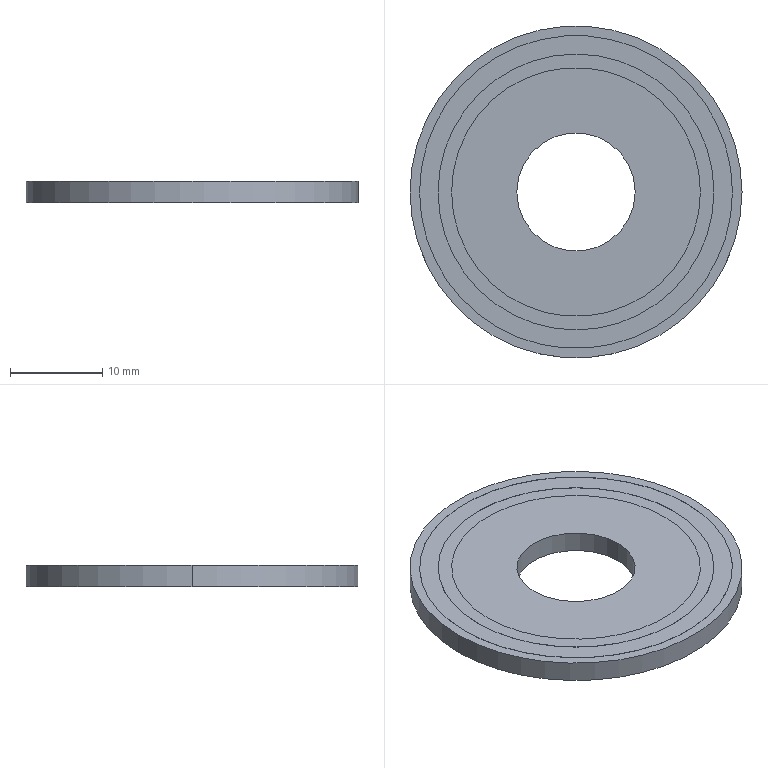Part | STEP file | 2 solids | 18 faces | box 35.9 x 35.9 x 2.3 mm | volume 2028 mm3 | cylinder 12 | plane 6 | commonest cylinder face diameters 26.9 x4 12.8 x2 29.83 x2 33.83 x2 35.9 x2
STEP:
#1=CARTESIAN_POINT('',(0.,0.,0.));
#2=DIRECTION('',(0.,0.,1.));
#3=DIRECTION('',(1.,0.,0.));
#4=AXIS2_PLACEMENT_3D('',#1,#2,#3);
#5=CARTESIAN_POINT('',(-13.45,0.,0.));
#6=VERTEX_POINT('',#5);
#7=CARTESIAN_POINT('',(-13.45,0.,2.3));
#8=VERTEX_POINT('',#7);
#9=CARTESIAN_POINT('',(-13.45,0.,-0.01));
#10=DIRECTION('',(0.,0.,1.));
#11=VECTOR('',#10,1.);
#12=LINE('',#9,#11);
#13=CARTESIAN_POINT('',(0.,0.,-0.01));
#14=DIRECTION('',(0.,0.,1.));
#15=DIRECTION('',(1.,0.,0.));
#16=AXIS2_PLACEMENT_3D('',#13,#14,#15);
#17=CYLINDRICAL_SURFACE('',#16,13.45);
#18=CARTESIAN_POINT('',(3.142,0.));
#19=DIRECTION('',(0.,1.));
#20=VECTOR('',#19,1.);
#21=LINE('',#18,#20);
#22=(GEOMETRIC_REPRESENTATION_CONTEXT(2)PARAMETRIC_REPRESENTATION_CONTEXT()REPRESENTATION_CONTEXT('',''));
#23=DEFINITIONAL_REPRESENTATION('',(#21),#22);
#24=PCURVE('',#17,#23);
#25=CARTESIAN_POINT('',(0.,0.,-0.01));
#26=DIRECTION('',(0.,0.,1.));
#27=DIRECTION('',(1.,0.,0.));
#28=AXIS2_PLACEMENT_3D('',#25,#26,#27);
#29=CYLINDRICAL_SURFACE('',#28,13.45);
#30=CARTESIAN_POINT('',(3.142,0.));
#31=DIRECTION('',(0.,1.));
#32=VECTOR('',#31,1.);
#33=LINE('',#30,#32);
#34=(GEOMETRIC_REPRESENTATION_CONTEXT(2)PARAMETRIC_REPRESENTATION_CONTEXT()REPRESENTATION_CONTEXT('',''));
#35=DEFINITIONAL_REPRESENTATION('',(#33),#34);
#36=PCURVE('',#29,#35);
#37=SURFACE_CURVE('',#12,(#24,#36),.PCURVE_S1.);
#38=EDGE_CURVE('',#6,#8,#37,.T.);
#39=ORIENTED_EDGE('',*,*,#38,.F.);
#40=CARTESIAN_POINT('',(13.45,0.,0.));
#41=VERTEX_POINT('',#40);
#42=CARTESIAN_POINT('',(0.,0.,0.));
#43=DIRECTION('',(0.,0.,1.));
#44=DIRECTION('',(1.,0.,0.));
#45=AXIS2_PLACEMENT_3D('',#42,#43,#44);
#46=CIRCLE('',#45,13.45);
#47=CARTESIAN_POINT('',(0.,0.01));
#48=DIRECTION('',(1.,0.));
#49=VECTOR('',#48,1.);
#50=LINE('',#47,#49);
#51=(GEOMETRIC_REPRESENTATION_CONTEXT(2)PARAMETRIC_REPRESENTATION_CONTEXT()REPRESENTATION_CONTEXT('',''));
#52=DEFINITIONAL_REPRESENTATION('',(#50),#51);
#53=PCURVE('',#17,#52);
#54=CARTESIAN_POINT('',(0.,0.,0.));
#55=DIRECTION('',(0.,0.,1.));
#56=DIRECTION('',(1.,0.,0.));
#57=AXIS2_PLACEMENT_3D('',#54,#55,#56);
#58=PLANE('',#57);
#59=CARTESIAN_POINT('',(0.,0.));
#60=DIRECTION('',(1.,0.));
#61=AXIS2_PLACEMENT_2D('',#59,#60);
#62=CIRCLE('',#61,13.45);
#63=(GEOMETRIC_REPRESENTATION_CONTEXT(2)PARAMETRIC_REPRESENTATION_CONTEXT()REPRESENTATION_CONTEXT('',''));
#64=DEFINITIONAL_REPRESENTATION('',(#62),#63);
#65=PCURVE('',#58,#64);
#66=SURFACE_CURVE('',#46,(#53,#65),.PCURVE_S1.);
#67=EDGE_CURVE('',#6,#41,#66,.T.);
#68=ORIENTED_EDGE('',*,*,#67,.T.);
#69=CARTESIAN_POINT('',(13.45,0.,2.3));
#70=VERTEX_POINT('',#69);
#71=CARTESIAN_POINT('',(13.45,0.,-0.01));
#72=DIRECTION('',(0.,0.,1.));
#73=VECTOR('',#72,1.);
#74=LINE('',#71,#73);
#75=CARTESIAN_POINT('',(6.283,0.));
#76=DIRECTION('',(0.,1.));
#77=VECTOR('',#76,1.);
#78=LINE('',#75,#77);
#79=(GEOMETRIC_REPRESENTATION_CONTEXT(2)PARAMETRIC_REPRESENTATION_CONTEXT()REPRESENTATION_CONTEXT('',''));
#80=DEFINITIONAL_REPRESENTATION('',(#78),#79);
#81=PCURVE('',#17,#80);
#82=CARTESIAN_POINT('',(0.,0.));
#83=DIRECTION('',(0.,1.));
#84=VECTOR('',#83,1.);
#85=LINE('',#82,#84);
#86=(GEOMETRIC_REPRESENTATION_CONTEXT(2)PARAMETRIC_REPRESENTATION_CONTEXT()REPRESENTATION_CONTEXT('',''));
#87=DEFINITIONAL_REPRESENTATION('',(#85),#86);
#88=PCURVE('',#29,#87);
#89=SURFACE_CURVE('',#74,(#81,#88),.PCURVE_S1.);
#90=EDGE_CURVE('',#41,#70,#89,.T.);
#91=ORIENTED_EDGE('',*,*,#90,.T.);
#92=CARTESIAN_POINT('',(0.,0.,2.3));
#93=DIRECTION('',(0.,0.,1.));
#94=DIRECTION('',(1.,0.,0.));
#95=AXIS2_PLACEMENT_3D('',#92,#93,#94);
#96=CIRCLE('',#95,13.45);
#97=CARTESIAN_POINT('',(0.,2.31));
#98=DIRECTION('',(1.,0.));
#99=VECTOR('',#98,1.);
#100=LINE('',#97,#99);
#101=(GEOMETRIC_REPRESENTATION_CONTEXT(2)PARAMETRIC_REPRESENTATION_CONTEXT()REPRESENTATION_CONTEXT('',''));
#102=DEFINITIONAL_REPRESENTATION('',(#100),#101);
#103=PCURVE('',#17,#102);
#104=CARTESIAN_POINT('',(0.,0.,2.3));
#105=DIRECTION('',(0.,0.,1.));
#106=DIRECTION('',(1.,0.,0.));
#107=AXIS2_PLACEMENT_3D('',#104,#105,#106);
#108=PLANE('',#107);
#109=CARTESIAN_POINT('',(0.,0.));
#110=DIRECTION('',(1.,0.));
#111=AXIS2_PLACEMENT_2D('',#109,#110);
#112=CIRCLE('',#111,13.45);
#113=(GEOMETRIC_REPRESENTATION_CONTEXT(2)PARAMETRIC_REPRESENTATION_CONTEXT()REPRESENTATION_CONTEXT('',''));
#114=DEFINITIONAL_REPRESENTATION('',(#112),#113);
#115=PCURVE('',#108,#114);
#116=SURFACE_CURVE('',#96,(#103,#115),.PCURVE_S1.);
#117=EDGE_CURVE('',#8,#70,#116,.T.);
#118=ORIENTED_EDGE('',*,*,#117,.F.);
#119=EDGE_LOOP('',(#39,#68,#91,#118));
#120=FACE_BOUND('',#119,.T.);
#121=ADVANCED_FACE('',(#120),#17,.T.);
#122=CARTESIAN_POINT('',(6.4,0.,0.));
#123=VERTEX_POINT('',#122);
#124=CARTESIAN_POINT('',(-6.4,0.,0.));
#125=VERTEX_POINT('',#124);
#126=CARTESIAN_POINT('',(0.,0.,0.));
#127=DIRECTION('',(0.,0.,1.));
#128=DIRECTION('',(1.,0.,0.));
#129=AXIS2_PLACEMENT_3D('',#126,#127,#128);
#130=CIRCLE('',#129,6.4);
#131=CARTESIAN_POINT('',(0.,0.,2.3));
#132=DIRECTION('',(0.,0.,-1.));
#133=DIRECTION('',(-1.,0.,0.));
#134=AXIS2_PLACEMENT_3D('',#131,#132,#133);
#135=CYLINDRICAL_SURFACE('',#134,6.4);
#136=CARTESIAN_POINT('',(3.142,2.3));
#137=DIRECTION('',(-1.,0.));
#138=VECTOR('',#137,1.);
#139=LINE('',#136,#138);
#140=(GEOMETRIC_REPRESENTATION_CONTEXT(2)PARAMETRIC_REPRESENTATION_CONTEXT()REPRESENTATION_CONTEXT('',''));
#141=DEFINITIONAL_REPRESENTATION('',(#139),#140);
#142=PCURVE('',#135,#141);
#143=CARTESIAN_POINT('',(0.,0.));
#144=DIRECTION('',(1.,0.));
#145=AXIS2_PLACEMENT_2D('',#143,#144);
#146=CIRCLE('',#145,6.4);
#147=(GEOMETRIC_REPRESENTATION_CONTEXT(2)PARAMETRIC_REPRESENTATION_CONTEXT()REPRESENTATION_CONTEXT('',''));
#148=DEFINITIONAL_REPRESENTATION('',(#146),#147);
#149=PCURVE('',#58,#148);
#150=SURFACE_CURVE('',#130,(#142,#149),.PCURVE_S1.);
#151=EDGE_CURVE('',#123,#125,#150,.T.);
#152=ORIENTED_EDGE('',*,*,#151,.T.);
#153=CARTESIAN_POINT('',(-6.4,0.,2.3));
#154=VERTEX_POINT('',#153);
#155=CARTESIAN_POINT('',(-6.4,0.,2.3));
#156=DIRECTION('',(0.,0.,-1.));
#157=VECTOR('',#156,1.);
#158=LINE('',#155,#157);
#159=CARTESIAN_POINT('',(0.,0.));
#160=DIRECTION('',(0.,1.));
#161=VECTOR('',#160,1.);
#162=LINE('',#159,#161);
#163=(GEOMETRIC_REPRESENTATION_CONTEXT(2)PARAMETRIC_REPRESENTATION_CONTEXT()REPRESENTATION_CONTEXT('',''));
#164=DEFINITIONAL_REPRESENTATION('',(#162),#163);
#165=PCURVE('',#135,#164);
#166=CARTESIAN_POINT('',(0.,0.,2.3));
#167=DIRECTION('',(0.,0.,-1.));
#168=DIRECTION('',(-1.,0.,0.));
#169=AXIS2_PLACEMENT_3D('',#166,#167,#168);
#170=CYLINDRICAL_SURFACE('',#169,6.4);
#171=CARTESIAN_POINT('',(6.283,0.));
#172=DIRECTION('',(0.,1.));
#173=VECTOR('',#172,1.);
#174=LINE('',#171,#173);
#175=(GEOMETRIC_REPRESENTATION_CONTEXT(2)PARAMETRIC_REPRESENTATION_CONTEXT()REPRESENTATION_CONTEXT('',''));
#176=DEFINITIONAL_REPRESENTATION('',(#174),#175);
#177=PCURVE('',#170,#176);
#178=SURFACE_CURVE('',#158,(#165,#177),.PCURVE_S1.);
#179=EDGE_CURVE('',#154,#125,#178,.T.);
#180=ORIENTED_EDGE('',*,*,#179,.F.);
#181=CARTESIAN_POINT('',(6.4,0.,2.3));
#182=VERTEX_POINT('',#181);
#183=CARTESIAN_POINT('',(0.,0.,2.3));
#184=DIRECTION('',(0.,0.,1.));
#185=DIRECTION('',(1.,0.,0.));
#186=AXIS2_PLACEMENT_3D('',#183,#184,#185);
#187=CIRCLE('',#186,6.4);
#188=CARTESIAN_POINT('',(3.142,0.));
#189=DIRECTION('',(-1.,0.));
#190=VECTOR('',#189,1.);
#191=LINE('',#188,#190);
#192=(GEOMETRIC_REPRESENTATION_CONTEXT(2)PARAMETRIC_REPRESENTATION_CONTEXT()REPRESENTATION_CONTEXT('',''));
#193=DEFINITIONAL_REPRESENTATION('',(#191),#192);
#194=PCURVE('',#135,#193);
#195=CARTESIAN_POINT('',(0.,0.));
#196=DIRECTION('',(1.,0.));
#197=AXIS2_PLACEMENT_2D('',#195,#196);
#198=CIRCLE('',#197,6.4);
#199=(GEOMETRIC_REPRESENTATION_CONTEXT(2)PARAMETRIC_REPRESENTATION_CONTEXT()REPRESENTATION_CONTEXT('',''));
#200=DEFINITIONAL_REPRESENTATION('',(#198),#199);
#201=PCURVE('',#108,#200);
#202=SURFACE_CURVE('',#187,(#194,#201),.PCURVE_S1.);
#203=EDGE_CURVE('',#182,#154,#202,.T.);
#204=ORIENTED_EDGE('',*,*,#203,.F.);
#205=CARTESIAN_POINT('',(6.4,0.,2.3));
#206=DIRECTION('',(0.,0.,-1.));
#207=VECTOR('',#206,1.);
#208=LINE('',#205,#207);
#209=CARTESIAN_POINT('',(3.142,0.));
#210=DIRECTION('',(0.,1.));
#211=VECTOR('',#210,1.);
#212=LINE('',#209,#211);
#213=(GEOMETRIC_REPRESENTATION_CONTEXT(2)PARAMETRIC_REPRESENTATION_CONTEXT()REPRESENTATION_CONTEXT('',''));
#214=DEFINITIONAL_REPRESENTATION('',(#212),#213);
#215=PCURVE('',#135,#214);
#216=CARTESIAN_POINT('',(3.142,0.));
#217=DIRECTION('',(0.,1.));
#218=VECTOR('',#217,1.);
#219=LINE('',#216,#218);
#220=(GEOMETRIC_REPRESENTATION_CONTEXT(2)PARAMETRIC_REPRESENTATION_CONTEXT()REPRESENTATION_CONTEXT('',''));
#221=DEFINITIONAL_REPRESENTATION('',(#219),#220);
#222=PCURVE('',#170,#221);
#223=SURFACE_CURVE('',#208,(#215,#222),.PCURVE_S1.);
#224=EDGE_CURVE('',#182,#123,#223,.T.);
#225=ORIENTED_EDGE('',*,*,#224,.T.);
#226=EDGE_LOOP('',(#152,#180,#204,#225));
#227=FACE_BOUND('',#226,.F.);
#228=ADVANCED_FACE('',(#227),#135,.F.);
#229=CARTESIAN_POINT('',(0.,0.,0.));
#230=DIRECTION('',(0.,0.,1.));
#231=DIRECTION('',(1.,0.,0.));
#232=AXIS2_PLACEMENT_3D('',#229,#230,#231);
#233=CIRCLE('',#232,13.45);
#234=CARTESIAN_POINT('',(0.,0.));
#235=DIRECTION('',(1.,0.));
#236=AXIS2_PLACEMENT_2D('',#234,#235);
#237=CIRCLE('',#236,13.45);
#238=(GEOMETRIC_REPRESENTATION_CONTEXT(2)PARAMETRIC_REPRESENTATION_CONTEXT()REPRESENTATION_CONTEXT('',''));
#239=DEFINITIONAL_REPRESENTATION('',(#237),#238);
#240=PCURVE('',#58,#239);
#241=CARTESIAN_POINT('',(0.,0.01));
#242=DIRECTION('',(1.,0.));
#243=VECTOR('',#242,1.);
#244=LINE('',#241,#243);
#245=(GEOMETRIC_REPRESENTATION_CONTEXT(2)PARAMETRIC_REPRESENTATION_CONTEXT()REPRESENTATION_CONTEXT('',''));
#246=DEFINITIONAL_REPRESENTATION('',(#244),#245);
#247=PCURVE('',#29,#246);
#248=SURFACE_CURVE('',#233,(#240,#247),.PCURVE_S1.);
#249=EDGE_CURVE('',#41,#6,#248,.T.);
#250=ORIENTED_EDGE('',*,*,#249,.F.);
#251=ORIENTED_EDGE('',*,*,#67,.F.);
#252=EDGE_LOOP('',(#250,#251));
#253=FACE_BOUND('',#252,.T.);
#254=CARTESIAN_POINT('',(0.,0.,0.));
#255=DIRECTION('',(0.,0.,1.));
#256=DIRECTION('',(1.,0.,0.));
#257=AXIS2_PLACEMENT_3D('',#254,#255,#256);
#258=CIRCLE('',#257,6.4);
#259=CARTESIAN_POINT('',(0.,0.));
#260=DIRECTION('',(1.,0.));
#261=AXIS2_PLACEMENT_2D('',#259,#260);
#262=CIRCLE('',#261,6.4);
#263=(GEOMETRIC_REPRESENTATION_CONTEXT(2)PARAMETRIC_REPRESENTATION_CONTEXT()REPRESENTATION_CONTEXT('',''));
#264=DEFINITIONAL_REPRESENTATION('',(#262),#263);
#265=PCURVE('',#58,#264);
#266=CARTESIAN_POINT('',(9.425,2.3));
#267=DIRECTION('',(-1.,0.));
#268=VECTOR('',#267,1.);
#269=LINE('',#266,#268);
#270=(GEOMETRIC_REPRESENTATION_CONTEXT(2)PARAMETRIC_REPRESENTATION_CONTEXT()REPRESENTATION_CONTEXT('',''));
#271=DEFINITIONAL_REPRESENTATION('',(#269),#270);
#272=PCURVE('',#170,#271);
#273=SURFACE_CURVE('',#258,(#265,#272),.PCURVE_S1.);
#274=EDGE_CURVE('',#125,#123,#273,.T.);
#275=ORIENTED_EDGE('',*,*,#274,.T.);
#276=ORIENTED_EDGE('',*,*,#151,.T.);
#277=EDGE_LOOP('',(#275,#276));
#278=FACE_BOUND('',#277,.T.);
#279=ADVANCED_FACE('',(#253,#278),#58,.F.);
#280=CARTESIAN_POINT('',(0.,0.,2.3));
#281=DIRECTION('',(0.,0.,1.));
#282=DIRECTION('',(1.,0.,0.));
#283=AXIS2_PLACEMENT_3D('',#280,#281,#282);
#284=CIRCLE('',#283,13.45);
#285=CARTESIAN_POINT('',(0.,0.));
#286=DIRECTION('',(1.,0.));
#287=AXIS2_PLACEMENT_2D('',#285,#286);
#288=CIRCLE('',#287,13.45);
#289=(GEOMETRIC_REPRESENTATION_CONTEXT(2)PARAMETRIC_REPRESENTATION_CONTEXT()REPRESENTATION_CONTEXT('',''));
#290=DEFINITIONAL_REPRESENTATION('',(#288),#289);
#291=PCURVE('',#108,#290);
#292=CARTESIAN_POINT('',(0.,2.31));
#293=DIRECTION('',(1.,0.));
#294=VECTOR('',#293,1.);
#295=LINE('',#292,#294);
#296=(GEOMETRIC_REPRESENTATION_CONTEXT(2)PARAMETRIC_REPRESENTATION_CONTEXT()REPRESENTATION_CONTEXT('',''));
#297=DEFINITIONAL_REPRESENTATION('',(#295),#296);
#298=PCURVE('',#29,#297);
#299=SURFACE_CURVE('',#284,(#291,#298),.PCURVE_S1.);
#300=EDGE_CURVE('',#70,#8,#299,.T.);
#301=ORIENTED_EDGE('',*,*,#300,.T.);
#302=ORIENTED_EDGE('',*,*,#117,.T.);
#303=EDGE_LOOP('',(#301,#302));
#304=FACE_BOUND('',#303,.T.);
#305=CARTESIAN_POINT('',(0.,0.,2.3));
#306=DIRECTION('',(0.,0.,1.));
#307=DIRECTION('',(1.,0.,0.));
#308=AXIS2_PLACEMENT_3D('',#305,#306,#307);
#309=CIRCLE('',#308,6.4);
#310=CARTESIAN_POINT('',(0.,0.));
#311=DIRECTION('',(1.,0.));
#312=AXIS2_PLACEMENT_2D('',#310,#311);
#313=CIRCLE('',#312,6.4);
#314=(GEOMETRIC_REPRESENTATION_CONTEXT(2)PARAMETRIC_REPRESENTATION_CONTEXT()REPRESENTATION_CONTEXT('',''));
#315=DEFINITIONAL_REPRESENTATION('',(#313),#314);
#316=PCURVE('',#108,#315);
#317=CARTESIAN_POINT('',(9.425,0.));
#318=DIRECTION('',(-1.,0.));
#319=VECTOR('',#318,1.);
#320=LINE('',#317,#319);
#321=(GEOMETRIC_REPRESENTATION_CONTEXT(2)PARAMETRIC_REPRESENTATION_CONTEXT()REPRESENTATION_CONTEXT('',''));
#322=DEFINITIONAL_REPRESENTATION('',(#320),#321);
#323=PCURVE('',#170,#322);
#324=SURFACE_CURVE('',#309,(#316,#323),.PCURVE_S1.);
#325=EDGE_CURVE('',#154,#182,#324,.T.);
#326=ORIENTED_EDGE('',*,*,#325,.F.);
#327=ORIENTED_EDGE('',*,*,#203,.F.);
#328=EDGE_LOOP('',(#326,#327));
#329=FACE_BOUND('',#328,.T.);
#330=ADVANCED_FACE('',(#304,#329),#108,.T.);
#331=ORIENTED_EDGE('',*,*,#249,.T.);
#332=ORIENTED_EDGE('',*,*,#38,.T.);
#333=ORIENTED_EDGE('',*,*,#300,.F.);
#334=ORIENTED_EDGE('',*,*,#90,.F.);
#335=EDGE_LOOP('',(#331,#332,#333,#334));
#336=FACE_BOUND('',#335,.T.);
#337=ADVANCED_FACE('',(#336),#29,.T.);
#338=ORIENTED_EDGE('',*,*,#179,.T.);
#339=ORIENTED_EDGE('',*,*,#274,.T.);
#340=ORIENTED_EDGE('',*,*,#224,.F.);
#341=ORIENTED_EDGE('',*,*,#325,.F.);
#342=EDGE_LOOP('',(#338,#339,#340,#341));
#343=FACE_BOUND('',#342,.F.);
#344=ADVANCED_FACE('',(#343),#170,.F.);
#345=CLOSED_SHELL('',(#121,#228,#279,#330,#337,#344));
#346=MANIFOLD_SOLID_BREP('',#345);
#347=CARTESIAN_POINT('',(-14.915,0.,2.28));
#348=VERTEX_POINT('',#347);
#349=CARTESIAN_POINT('',(-14.915,0.,2.3));
#350=VERTEX_POINT('',#349);
#351=CARTESIAN_POINT('',(-14.915,0.,2.28));
#352=DIRECTION('',(0.,0.,1.));
#353=VECTOR('',#352,1.);
#354=LINE('',#351,#353);
#355=CARTESIAN_POINT('',(0.,0.,2.28));
#356=DIRECTION('',(0.,0.,1.));
#357=DIRECTION('',(1.,0.,0.));
#358=AXIS2_PLACEMENT_3D('',#355,#356,#357);
#359=CYLINDRICAL_SURFACE('',#358,14.915);
#360=CARTESIAN_POINT('',(3.142,0.));
#361=DIRECTION('',(0.,1.));
#362=VECTOR('',#361,1.);
#363=LINE('',#360,#362);
#364=(GEOMETRIC_REPRESENTATION_CONTEXT(2)PARAMETRIC_REPRESENTATION_CONTEXT()REPRESENTATION_CONTEXT('',''));
#365=DEFINITIONAL_REPRESENTATION('',(#363),#364);
#366=PCURVE('',#359,#365);
#367=CARTESIAN_POINT('',(0.,0.,2.28));
#368=DIRECTION('',(0.,0.,1.));
#369=DIRECTION('',(1.,0.,0.));
#370=AXIS2_PLACEMENT_3D('',#367,#368,#369);
#371=CYLINDRICAL_SURFACE('',#370,14.915);
#372=CARTESIAN_POINT('',(3.142,0.));
#373=DIRECTION('',(0.,1.));
#374=VECTOR('',#373,1.);
#375=LINE('',#372,#374);
#376=(GEOMETRIC_REPRESENTATION_CONTEXT(2)PARAMETRIC_REPRESENTATION_CONTEXT()REPRESENTATION_CONTEXT('',''));
#377=DEFINITIONAL_REPRESENTATION('',(#375),#376);
#378=PCURVE('',#371,#377);
#379=SURFACE_CURVE('',#354,(#366,#378),.PCURVE_S1.);
#380=EDGE_CURVE('',#348,#350,#379,.T.);
#381=ORIENTED_EDGE('',*,*,#380,.F.);
#382=CARTESIAN_POINT('',(14.915,0.,2.28));
#383=VERTEX_POINT('',#382);
#384=CARTESIAN_POINT('',(0.,0.,2.28));
#385=DIRECTION('',(0.,0.,1.));
#386=DIRECTION('',(1.,0.,0.));
#387=AXIS2_PLACEMENT_3D('',#384,#385,#386);
#388=CIRCLE('',#387,14.915);
#389=CARTESIAN_POINT('',(0.,0.));
#390=DIRECTION('',(1.,0.));
#391=VECTOR('',#390,1.);
#392=LINE('',#389,#391);
#393=(GEOMETRIC_REPRESENTATION_CONTEXT(2)PARAMETRIC_REPRESENTATION_CONTEXT()REPRESENTATION_CONTEXT('',''));
#394=DEFINITIONAL_REPRESENTATION('',(#392),#393);
#395=PCURVE('',#359,#394);
#396=CARTESIAN_POINT('',(0.,0.,2.28));
#397=DIRECTION('',(0.,0.,1.));
#398=DIRECTION('',(1.,0.,0.));
#399=AXIS2_PLACEMENT_3D('',#396,#397,#398);
#400=PLANE('',#399);
#401=CARTESIAN_POINT('',(0.,0.));
#402=DIRECTION('',(1.,0.));
#403=AXIS2_PLACEMENT_2D('',#401,#402);
#404=CIRCLE('',#403,14.915);
#405=(GEOMETRIC_REPRESENTATION_CONTEXT(2)PARAMETRIC_REPRESENTATION_CONTEXT()REPRESENTATION_CONTEXT('',''));
#406=DEFINITIONAL_REPRESENTATION('',(#404),#405);
#407=PCURVE('',#400,#406);
#408=SURFACE_CURVE('',#388,(#395,#407),.PCURVE_S1.);
#409=EDGE_CURVE('',#348,#383,#408,.T.);
#410=ORIENTED_EDGE('',*,*,#409,.T.);
#411=CARTESIAN_POINT('',(14.915,0.,2.3));
#412=VERTEX_POINT('',#411);
#413=CARTESIAN_POINT('',(14.915,0.,2.28));
#414=DIRECTION('',(0.,0.,1.));
#415=VECTOR('',#414,1.);
#416=LINE('',#413,#415);
#417=CARTESIAN_POINT('',(6.283,0.));
#418=DIRECTION('',(0.,1.));
#419=VECTOR('',#418,1.);
#420=LINE('',#417,#419);
#421=(GEOMETRIC_REPRESENTATION_CONTEXT(2)PARAMETRIC_REPRESENTATION_CONTEXT()REPRESENTATION_CONTEXT('',''));
#422=DEFINITIONAL_REPRESENTATION('',(#420),#421);
#423=PCURVE('',#359,#422);
#424=CARTESIAN_POINT('',(0.,0.));
#425=DIRECTION('',(0.,1.));
#426=VECTOR('',#425,1.);
#427=LINE('',#424,#426);
#428=(GEOMETRIC_REPRESENTATION_CONTEXT(2)PARAMETRIC_REPRESENTATION_CONTEXT()REPRESENTATION_CONTEXT('',''));
#429=DEFINITIONAL_REPRESENTATION('',(#427),#428);
#430=PCURVE('',#371,#429);
#431=SURFACE_CURVE('',#416,(#423,#430),.PCURVE_S1.);
#432=EDGE_CURVE('',#383,#412,#431,.T.);
#433=ORIENTED_EDGE('',*,*,#432,.T.);
#434=CARTESIAN_POINT('',(0.,0.,2.3));
#435=DIRECTION('',(0.,0.,1.));
#436=DIRECTION('',(1.,0.,0.));
#437=AXIS2_PLACEMENT_3D('',#434,#435,#436);
#438=CIRCLE('',#437,14.915);
#439=CARTESIAN_POINT('',(0.,0.02));
#440=DIRECTION('',(1.,0.));
#441=VECTOR('',#440,1.);
#442=LINE('',#439,#441);
#443=(GEOMETRIC_REPRESENTATION_CONTEXT(2)PARAMETRIC_REPRESENTATION_CONTEXT()REPRESENTATION_CONTEXT('',''));
#444=DEFINITIONAL_REPRESENTATION('',(#442),#443);
#445=PCURVE('',#359,#444);
#446=CARTESIAN_POINT('',(0.,0.,2.3));
#447=DIRECTION('',(0.,0.,1.));
#448=DIRECTION('',(1.,0.,0.));
#449=AXIS2_PLACEMENT_3D('',#446,#447,#448);
#450=PLANE('',#449);
#451=CARTESIAN_POINT('',(0.,0.));
#452=DIRECTION('',(1.,0.));
#453=AXIS2_PLACEMENT_2D('',#451,#452);
#454=CIRCLE('',#453,14.915);
#455=(GEOMETRIC_REPRESENTATION_CONTEXT(2)PARAMETRIC_REPRESENTATION_CONTEXT()REPRESENTATION_CONTEXT('',''));
#456=DEFINITIONAL_REPRESENTATION('',(#454),#455);
#457=PCURVE('',#450,#456);
#458=SURFACE_CURVE('',#438,(#445,#457),.PCURVE_S1.);
#459=EDGE_CURVE('',#350,#412,#458,.T.);
#460=ORIENTED_EDGE('',*,*,#459,.F.);
#461=EDGE_LOOP('',(#381,#410,#433,#460));
#462=FACE_BOUND('',#461,.T.);
#463=ADVANCED_FACE('',(#462),#359,.T.);
#464=CARTESIAN_POINT('',(16.915,0.,2.28));
#465=VERTEX_POINT('',#464);
#466=CARTESIAN_POINT('',(-16.915,0.,2.28));
#467=VERTEX_POINT('',#466);
#468=CARTESIAN_POINT('',(0.,0.,2.28));
#469=DIRECTION('',(0.,0.,1.));
#470=DIRECTION('',(1.,0.,0.));
#471=AXIS2_PLACEMENT_3D('',#468,#469,#470);
#472=CIRCLE('',#471,16.915);
#473=CARTESIAN_POINT('',(0.,0.));
#474=DIRECTION('',(1.,0.));
#475=AXIS2_PLACEMENT_2D('',#473,#474);
#476=CIRCLE('',#475,16.915);
#477=(GEOMETRIC_REPRESENTATION_CONTEXT(2)PARAMETRIC_REPRESENTATION_CONTEXT()REPRESENTATION_CONTEXT('',''));
#478=DEFINITIONAL_REPRESENTATION('',(#476),#477);
#479=PCURVE('',#400,#478);
#480=CARTESIAN_POINT('',(0.,0.,2.28));
#481=DIRECTION('',(0.,0.,1.));
#482=DIRECTION('',(1.,0.,0.));
#483=AXIS2_PLACEMENT_3D('',#480,#481,#482);
#484=CYLINDRICAL_SURFACE('',#483,16.915);
#485=CARTESIAN_POINT('',(0.,0.));
#486=DIRECTION('',(1.,0.));
#487=VECTOR('',#486,1.);
#488=LINE('',#485,#487);
#489=(GEOMETRIC_REPRESENTATION_CONTEXT(2)PARAMETRIC_REPRESENTATION_CONTEXT()REPRESENTATION_CONTEXT('',''));
#490=DEFINITIONAL_REPRESENTATION('',(#488),#489);
#491=PCURVE('',#484,#490);
#492=SURFACE_CURVE('',#472,(#479,#491),.PCURVE_S1.);
#493=EDGE_CURVE('',#465,#467,#492,.T.);
#494=ORIENTED_EDGE('',*,*,#493,.T.);
#495=CARTESIAN_POINT('',(0.,0.,2.28));
#496=DIRECTION('',(0.,0.,1.));
#497=DIRECTION('',(1.,0.,0.));
#498=AXIS2_PLACEMENT_3D('',#495,#496,#497);
#499=CIRCLE('',#498,16.915);
#500=CARTESIAN_POINT('',(0.,0.));
#501=DIRECTION('',(1.,0.));
#502=AXIS2_PLACEMENT_2D('',#500,#501);
#503=CIRCLE('',#502,16.915);
#504=(GEOMETRIC_REPRESENTATION_CONTEXT(2)PARAMETRIC_REPRESENTATION_CONTEXT()REPRESENTATION_CONTEXT('',''));
#505=DEFINITIONAL_REPRESENTATION('',(#503),#504);
#506=PCURVE('',#400,#505);
#507=CARTESIAN_POINT('',(0.,0.,2.28));
#508=DIRECTION('',(0.,0.,1.));
#509=DIRECTION('',(1.,0.,0.));
#510=AXIS2_PLACEMENT_3D('',#507,#508,#509);
#511=CYLINDRICAL_SURFACE('',#510,16.915);
#512=CARTESIAN_POINT('',(0.,0.));
#513=DIRECTION('',(1.,0.));
#514=VECTOR('',#513,1.);
#515=LINE('',#512,#514);
#516=(GEOMETRIC_REPRESENTATION_CONTEXT(2)PARAMETRIC_REPRESENTATION_CONTEXT()REPRESENTATION_CONTEXT('',''));
#517=DEFINITIONAL_REPRESENTATION('',(#515),#516);
#518=PCURVE('',#511,#517);
#519=SURFACE_CURVE('',#499,(#506,#518),.PCURVE_S1.);
#520=EDGE_CURVE('',#467,#465,#519,.T.);
#521=ORIENTED_EDGE('',*,*,#520,.T.);
#522=EDGE_LOOP('',(#494,#521));
#523=FACE_BOUND('',#522,.T.);
#524=CARTESIAN_POINT('',(0.,0.,2.28));
#525=DIRECTION('',(0.,0.,1.));
#526=DIRECTION('',(1.,0.,0.));
#527=AXIS2_PLACEMENT_3D('',#524,#525,#526);
#528=CIRCLE('',#527,14.915);
#529=CARTESIAN_POINT('',(0.,0.));
#530=DIRECTION('',(1.,0.));
#531=AXIS2_PLACEMENT_2D('',#529,#530);
#532=CIRCLE('',#531,14.915);
#533=(GEOMETRIC_REPRESENTATION_CONTEXT(2)PARAMETRIC_REPRESENTATION_CONTEXT()REPRESENTATION_CONTEXT('',''));
#534=DEFINITIONAL_REPRESENTATION('',(#532),#533);
#535=PCURVE('',#400,#534);
#536=CARTESIAN_POINT('',(0.,0.));
#537=DIRECTION('',(1.,0.));
#538=VECTOR('',#537,1.);
#539=LINE('',#536,#538);
#540=(GEOMETRIC_REPRESENTATION_CONTEXT(2)PARAMETRIC_REPRESENTATION_CONTEXT()REPRESENTATION_CONTEXT('',''));
#541=DEFINITIONAL_REPRESENTATION('',(#539),#540);
#542=PCURVE('',#371,#541);
#543=SURFACE_CURVE('',#528,(#535,#542),.PCURVE_S1.);
#544=EDGE_CURVE('',#383,#348,#543,.T.);
#545=ORIENTED_EDGE('',*,*,#544,.F.);
#546=ORIENTED_EDGE('',*,*,#409,.F.);
#547=EDGE_LOOP('',(#545,#546));
#548=FACE_BOUND('',#547,.T.);
#549=ADVANCED_FACE('',(#523,#548),#400,.T.);
#550=CARTESIAN_POINT('',(16.915,0.,2.3));
#551=VERTEX_POINT('',#550);
#552=CARTESIAN_POINT('',(-16.915,0.,2.3));
#553=VERTEX_POINT('',#552);
#554=CARTESIAN_POINT('',(0.,0.,2.3));
#555=DIRECTION('',(0.,0.,1.));
#556=DIRECTION('',(1.,0.,0.));
#557=AXIS2_PLACEMENT_3D('',#554,#555,#556);
#558=CIRCLE('',#557,16.915);
#559=CARTESIAN_POINT('',(0.,0.02));
#560=DIRECTION('',(1.,0.));
#561=VECTOR('',#560,1.);
#562=LINE('',#559,#561);
#563=(GEOMETRIC_REPRESENTATION_CONTEXT(2)PARAMETRIC_REPRESENTATION_CONTEXT()REPRESENTATION_CONTEXT('',''));
#564=DEFINITIONAL_REPRESENTATION('',(#562),#563);
#565=PCURVE('',#484,#564);
#566=CARTESIAN_POINT('',(0.,0.,2.3));
#567=DIRECTION('',(0.,0.,1.));
#568=DIRECTION('',(1.,0.,0.));
#569=AXIS2_PLACEMENT_3D('',#566,#567,#568);
#570=PLANE('',#569);
#571=CARTESIAN_POINT('',(0.,0.));
#572=DIRECTION('',(1.,0.));
#573=AXIS2_PLACEMENT_2D('',#571,#572);
#574=CIRCLE('',#573,16.915);
#575=(GEOMETRIC_REPRESENTATION_CONTEXT(2)PARAMETRIC_REPRESENTATION_CONTEXT()REPRESENTATION_CONTEXT('',''));
#576=DEFINITIONAL_REPRESENTATION('',(#574),#575);
#577=PCURVE('',#570,#576);
#578=SURFACE_CURVE('',#558,(#565,#577),.PCURVE_S1.);
#579=EDGE_CURVE('',#551,#553,#578,.T.);
#580=ORIENTED_EDGE('',*,*,#579,.F.);
#581=CARTESIAN_POINT('',(16.915,0.,2.28));
#582=DIRECTION('',(0.,0.,1.));
#583=VECTOR('',#582,1.);
#584=LINE('',#581,#583);
#585=CARTESIAN_POINT('',(0.,0.));
#586=DIRECTION('',(0.,1.));
#587=VECTOR('',#586,1.);
#588=LINE('',#585,#587);
#589=(GEOMETRIC_REPRESENTATION_CONTEXT(2)PARAMETRIC_REPRESENTATION_CONTEXT()REPRESENTATION_CONTEXT('',''));
#590=DEFINITIONAL_REPRESENTATION('',(#588),#589);
#591=PCURVE('',#484,#590);
#592=CARTESIAN_POINT('',(6.283,0.));
#593=DIRECTION('',(0.,1.));
#594=VECTOR('',#593,1.);
#595=LINE('',#592,#594);
#596=(GEOMETRIC_REPRESENTATION_CONTEXT(2)PARAMETRIC_REPRESENTATION_CONTEXT()REPRESENTATION_CONTEXT('',''));
#597=DEFINITIONAL_REPRESENTATION('',(#595),#596);
#598=PCURVE('',#511,#597);
#599=SURFACE_CURVE('',#584,(#591,#598),.PCURVE_S1.);
#600=EDGE_CURVE('',#465,#551,#599,.T.);
#601=ORIENTED_EDGE('',*,*,#600,.F.);
#602=ORIENTED_EDGE('',*,*,#493,.T.);
#603=CARTESIAN_POINT('',(-16.915,0.,2.28));
#604=DIRECTION('',(0.,0.,1.));
#605=VECTOR('',#604,1.);
#606=LINE('',#603,#605);
#607=CARTESIAN_POINT('',(3.142,0.));
#608=DIRECTION('',(0.,1.));
#609=VECTOR('',#608,1.);
#610=LINE('',#607,#609);
#611=(GEOMETRIC_REPRESENTATION_CONTEXT(2)PARAMETRIC_REPRESENTATION_CONTEXT()REPRESENTATION_CONTEXT('',''));
#612=DEFINITIONAL_REPRESENTATION('',(#610),#611);
#613=PCURVE('',#484,#612);
#614=CARTESIAN_POINT('',(3.142,0.));
#615=DIRECTION('',(0.,1.));
#616=VECTOR('',#615,1.);
#617=LINE('',#614,#616);
#618=(GEOMETRIC_REPRESENTATION_CONTEXT(2)PARAMETRIC_REPRESENTATION_CONTEXT()REPRESENTATION_CONTEXT('',''));
#619=DEFINITIONAL_REPRESENTATION('',(#617),#618);
#620=PCURVE('',#511,#619);
#621=SURFACE_CURVE('',#606,(#613,#620),.PCURVE_S1.);
#622=EDGE_CURVE('',#467,#553,#621,.T.);
#623=ORIENTED_EDGE('',*,*,#622,.T.);
#624=EDGE_LOOP('',(#580,#601,#602,#623));
#625=FACE_BOUND('',#624,.F.);
#626=ADVANCED_FACE('',(#625),#484,.F.);
#627=CARTESIAN_POINT('',(17.95,0.,2.3));
#628=VERTEX_POINT('',#627);
#629=CARTESIAN_POINT('',(17.95,0.,0.));
#630=VERTEX_POINT('',#629);
#631=CARTESIAN_POINT('',(17.95,0.,2.3));
#632=DIRECTION('',(0.,0.,-1.));
#633=VECTOR('',#632,1.);
#634=LINE('',#631,#633);
#635=CARTESIAN_POINT('',(0.,0.,2.3));
#636=DIRECTION('',(0.,0.,-1.));
#637=DIRECTION('',(-1.,0.,0.));
#638=AXIS2_PLACEMENT_3D('',#635,#636,#637);
#639=CYLINDRICAL_SURFACE('',#638,17.95);
#640=CARTESIAN_POINT('',(3.142,0.));
#641=DIRECTION('',(0.,1.));
#642=VECTOR('',#641,1.);
#643=LINE('',#640,#642);
#644=(GEOMETRIC_REPRESENTATION_CONTEXT(2)PARAMETRIC_REPRESENTATION_CONTEXT()REPRESENTATION_CONTEXT('',''));
#645=DEFINITIONAL_REPRESENTATION('',(#643),#644);
#646=PCURVE('',#639,#645);
#647=CARTESIAN_POINT('',(0.,0.,2.3));
#648=DIRECTION('',(0.,0.,-1.));
#649=DIRECTION('',(-1.,0.,0.));
#650=AXIS2_PLACEMENT_3D('',#647,#648,#649);
#651=CYLINDRICAL_SURFACE('',#650,17.95);
#652=CARTESIAN_POINT('',(3.142,0.));
#653=DIRECTION('',(0.,1.));
#654=VECTOR('',#653,1.);
#655=LINE('',#652,#654);
#656=(GEOMETRIC_REPRESENTATION_CONTEXT(2)PARAMETRIC_REPRESENTATION_CONTEXT()REPRESENTATION_CONTEXT('',''));
#657=DEFINITIONAL_REPRESENTATION('',(#655),#656);
#658=PCURVE('',#651,#657);
#659=SURFACE_CURVE('',#634,(#646,#658),.PCURVE_S1.);
#660=EDGE_CURVE('',#628,#630,#659,.T.);
#661=ORIENTED_EDGE('',*,*,#660,.F.);
#662=CARTESIAN_POINT('',(-17.95,0.,2.3));
#663=VERTEX_POINT('',#662);
#664=CARTESIAN_POINT('',(0.,0.,2.3));
#665=DIRECTION('',(0.,0.,1.));
#666=DIRECTION('',(1.,0.,0.));
#667=AXIS2_PLACEMENT_3D('',#664,#665,#666);
#668=CIRCLE('',#667,17.95);
#669=CARTESIAN_POINT('',(9.425,0.));
#670=DIRECTION('',(-1.,0.));
#671=VECTOR('',#670,1.);
#672=LINE('',#669,#671);
#673=(GEOMETRIC_REPRESENTATION_CONTEXT(2)PARAMETRIC_REPRESENTATION_CONTEXT()REPRESENTATION_CONTEXT('',''));
#674=DEFINITIONAL_REPRESENTATION('',(#672),#673);
#675=PCURVE('',#639,#674);
#676=CARTESIAN_POINT('',(0.,0.));
#677=DIRECTION('',(1.,0.));
#678=AXIS2_PLACEMENT_2D('',#676,#677);
#679=CIRCLE('',#678,17.95);
#680=(GEOMETRIC_REPRESENTATION_CONTEXT(2)PARAMETRIC_REPRESENTATION_CONTEXT()REPRESENTATION_CONTEXT('',''));
#681=DEFINITIONAL_REPRESENTATION('',(#679),#680);
#682=PCURVE('',#570,#681);
#683=SURFACE_CURVE('',#668,(#675,#682),.PCURVE_S1.);
#684=EDGE_CURVE('',#663,#628,#683,.T.);
#685=ORIENTED_EDGE('',*,*,#684,.F.);
#686=CARTESIAN_POINT('',(-17.95,0.,0.));
#687=VERTEX_POINT('',#686);
#688=CARTESIAN_POINT('',(-17.95,0.,2.3));
#689=DIRECTION('',(0.,0.,-1.));
#690=VECTOR('',#689,1.);
#691=LINE('',#688,#690);
#692=CARTESIAN_POINT('',(6.283,0.));
#693=DIRECTION('',(0.,1.));
#694=VECTOR('',#693,1.);
#695=LINE('',#692,#694);
#696=(GEOMETRIC_REPRESENTATION_CONTEXT(2)PARAMETRIC_REPRESENTATION_CONTEXT()REPRESENTATION_CONTEXT('',''));
#697=DEFINITIONAL_REPRESENTATION('',(#695),#696);
#698=PCURVE('',#639,#697);
#699=CARTESIAN_POINT('',(0.,0.));
#700=DIRECTION('',(0.,1.));
#701=VECTOR('',#700,1.);
#702=LINE('',#699,#701);
#703=(GEOMETRIC_REPRESENTATION_CONTEXT(2)PARAMETRIC_REPRESENTATION_CONTEXT()REPRESENTATION_CONTEXT('',''));
#704=DEFINITIONAL_REPRESENTATION('',(#702),#703);
#705=PCURVE('',#651,#704);
#706=SURFACE_CURVE('',#691,(#698,#705),.PCURVE_S1.);
#707=EDGE_CURVE('',#663,#687,#706,.T.);
#708=ORIENTED_EDGE('',*,*,#707,.T.);
#709=CARTESIAN_POINT('',(0.,0.,0.));
#710=DIRECTION('',(0.,0.,1.));
#711=DIRECTION('',(1.,0.,0.));
#712=AXIS2_PLACEMENT_3D('',#709,#710,#711);
#713=CIRCLE('',#712,17.95);
#714=CARTESIAN_POINT('',(9.425,2.3));
#715=DIRECTION('',(-1.,0.));
#716=VECTOR('',#715,1.);
#717=LINE('',#714,#716);
#718=(GEOMETRIC_REPRESENTATION_CONTEXT(2)PARAMETRIC_REPRESENTATION_CONTEXT()REPRESENTATION_CONTEXT('',''));
#719=DEFINITIONAL_REPRESENTATION('',(#717),#718);
#720=PCURVE('',#639,#719);
#721=CARTESIAN_POINT('',(0.,0.,0.));
#722=DIRECTION('',(0.,0.,1.));
#723=DIRECTION('',(1.,0.,0.));
#724=AXIS2_PLACEMENT_3D('',#721,#722,#723);
#725=PLANE('',#724);
#726=CARTESIAN_POINT('',(0.,0.));
#727=DIRECTION('',(1.,0.));
#728=AXIS2_PLACEMENT_2D('',#726,#727);
#729=CIRCLE('',#728,17.95);
#730=(GEOMETRIC_REPRESENTATION_CONTEXT(2)PARAMETRIC_REPRESENTATION_CONTEXT()REPRESENTATION_CONTEXT('',''));
#731=DEFINITIONAL_REPRESENTATION('',(#729),#730);
#732=PCURVE('',#725,#731);
#733=SURFACE_CURVE('',#713,(#720,#732),.PCURVE_S1.);
#734=EDGE_CURVE('',#687,#630,#733,.T.);
#735=ORIENTED_EDGE('',*,*,#734,.T.);
#736=EDGE_LOOP('',(#661,#685,#708,#735));
#737=FACE_BOUND('',#736,.T.);
#738=ADVANCED_FACE('',(#737),#639,.T.);
#739=ORIENTED_EDGE('',*,*,#734,.F.);
#740=CARTESIAN_POINT('',(0.,0.,0.));
#741=DIRECTION('',(0.,0.,1.));
#742=DIRECTION('',(1.,0.,0.));
#743=AXIS2_PLACEMENT_3D('',#740,#741,#742);
#744=CIRCLE('',#743,17.95);
#745=CARTESIAN_POINT('',(0.,0.));
#746=DIRECTION('',(1.,0.));
#747=AXIS2_PLACEMENT_2D('',#745,#746);
#748=CIRCLE('',#747,17.95);
#749=(GEOMETRIC_REPRESENTATION_CONTEXT(2)PARAMETRIC_REPRESENTATION_CONTEXT()REPRESENTATION_CONTEXT('',''));
#750=DEFINITIONAL_REPRESENTATION('',(#748),#749);
#751=PCURVE('',#725,#750);
#752=CARTESIAN_POINT('',(3.142,2.3));
#753=DIRECTION('',(-1.,0.));
#754=VECTOR('',#753,1.);
#755=LINE('',#752,#754);
#756=(GEOMETRIC_REPRESENTATION_CONTEXT(2)PARAMETRIC_REPRESENTATION_CONTEXT()REPRESENTATION_CONTEXT('',''));
#757=DEFINITIONAL_REPRESENTATION('',(#755),#756);
#758=PCURVE('',#651,#757);
#759=SURFACE_CURVE('',#744,(#751,#758),.PCURVE_S1.);
#760=EDGE_CURVE('',#630,#687,#759,.T.);
#761=ORIENTED_EDGE('',*,*,#760,.F.);
#762=EDGE_LOOP('',(#739,#761));
#763=FACE_BOUND('',#762,.T.);
#764=CARTESIAN_POINT('',(13.45,0.,0.));
#765=VERTEX_POINT('',#764);
#766=CARTESIAN_POINT('',(-13.45,0.,0.));
#767=VERTEX_POINT('',#766);
#768=CARTESIAN_POINT('',(0.,0.,0.));
#769=DIRECTION('',(0.,0.,1.));
#770=DIRECTION('',(1.,0.,0.));
#771=AXIS2_PLACEMENT_3D('',#768,#769,#770);
#772=CIRCLE('',#771,13.45);
#773=CARTESIAN_POINT('',(0.,0.));
#774=DIRECTION('',(1.,0.));
#775=AXIS2_PLACEMENT_2D('',#773,#774);
#776=CIRCLE('',#775,13.45);
#777=(GEOMETRIC_REPRESENTATION_CONTEXT(2)PARAMETRIC_REPRESENTATION_CONTEXT()REPRESENTATION_CONTEXT('',''));
#778=DEFINITIONAL_REPRESENTATION('',(#776),#777);
#779=PCURVE('',#725,#778);
#780=CARTESIAN_POINT('',(0.,0.,-0.01));
#781=DIRECTION('',(0.,0.,1.));
#782=DIRECTION('',(1.,0.,0.));
#783=AXIS2_PLACEMENT_3D('',#780,#781,#782);
#784=CYLINDRICAL_SURFACE('',#783,13.45);
#785=CARTESIAN_POINT('',(0.,0.01));
#786=DIRECTION('',(1.,0.));
#787=VECTOR('',#786,1.);
#788=LINE('',#785,#787);
#789=(GEOMETRIC_REPRESENTATION_CONTEXT(2)PARAMETRIC_REPRESENTATION_CONTEXT()REPRESENTATION_CONTEXT('',''));
#790=DEFINITIONAL_REPRESENTATION('',(#788),#789);
#791=PCURVE('',#784,#790);
#792=SURFACE_CURVE('',#772,(#779,#791),.PCURVE_S1.);
#793=EDGE_CURVE('',#765,#767,#792,.T.);
#794=ORIENTED_EDGE('',*,*,#793,.T.);
#795=CARTESIAN_POINT('',(0.,0.,0.));
#796=DIRECTION('',(0.,0.,1.));
#797=DIRECTION('',(1.,0.,0.));
#798=AXIS2_PLACEMENT_3D('',#795,#796,#797);
#799=CIRCLE('',#798,13.45);
#800=CARTESIAN_POINT('',(0.,0.));
#801=DIRECTION('',(1.,0.));
#802=AXIS2_PLACEMENT_2D('',#800,#801);
#803=CIRCLE('',#802,13.45);
#804=(GEOMETRIC_REPRESENTATION_CONTEXT(2)PARAMETRIC_REPRESENTATION_CONTEXT()REPRESENTATION_CONTEXT('',''));
#805=DEFINITIONAL_REPRESENTATION('',(#803),#804);
#806=PCURVE('',#725,#805);
#807=CARTESIAN_POINT('',(0.,0.,-0.01));
#808=DIRECTION('',(0.,0.,1.));
#809=DIRECTION('',(1.,0.,0.));
#810=AXIS2_PLACEMENT_3D('',#807,#808,#809);
#811=CYLINDRICAL_SURFACE('',#810,13.45);
#812=CARTESIAN_POINT('',(0.,0.01));
#813=DIRECTION('',(1.,0.));
#814=VECTOR('',#813,1.);
#815=LINE('',#812,#814);
#816=(GEOMETRIC_REPRESENTATION_CONTEXT(2)PARAMETRIC_REPRESENTATION_CONTEXT()REPRESENTATION_CONTEXT('',''));
#817=DEFINITIONAL_REPRESENTATION('',(#815),#816);
#818=PCURVE('',#811,#817);
#819=SURFACE_CURVE('',#799,(#806,#818),.PCURVE_S1.);
#820=EDGE_CURVE('',#767,#765,#819,.T.);
#821=ORIENTED_EDGE('',*,*,#820,.T.);
#822=EDGE_LOOP('',(#794,#821));
#823=FACE_BOUND('',#822,.T.);
#824=ADVANCED_FACE('',(#763,#823),#725,.F.);
#825=ORIENTED_EDGE('',*,*,#684,.T.);
#826=CARTESIAN_POINT('',(0.,0.,2.3));
#827=DIRECTION('',(0.,0.,1.));
#828=DIRECTION('',(1.,0.,0.));
#829=AXIS2_PLACEMENT_3D('',#826,#827,#828);
#830=CIRCLE('',#829,17.95);
#831=CARTESIAN_POINT('',(0.,0.));
#832=DIRECTION('',(1.,0.));
#833=AXIS2_PLACEMENT_2D('',#831,#832);
#834=CIRCLE('',#833,17.95);
#835=(GEOMETRIC_REPRESENTATION_CONTEXT(2)PARAMETRIC_REPRESENTATION_CONTEXT()REPRESENTATION_CONTEXT('',''));
#836=DEFINITIONAL_REPRESENTATION('',(#834),#835);
#837=PCURVE('',#570,#836);
#838=CARTESIAN_POINT('',(3.142,0.));
#839=DIRECTION('',(-1.,0.));
#840=VECTOR('',#839,1.);
#841=LINE('',#838,#840);
#842=(GEOMETRIC_REPRESENTATION_CONTEXT(2)PARAMETRIC_REPRESENTATION_CONTEXT()REPRESENTATION_CONTEXT('',''));
#843=DEFINITIONAL_REPRESENTATION('',(#841),#842);
#844=PCURVE('',#651,#843);
#845=SURFACE_CURVE('',#830,(#837,#844),.PCURVE_S1.);
#846=EDGE_CURVE('',#628,#663,#845,.T.);
#847=ORIENTED_EDGE('',*,*,#846,.T.);
#848=EDGE_LOOP('',(#825,#847));
#849=FACE_BOUND('',#848,.T.);
#850=ORIENTED_EDGE('',*,*,#579,.F.);
#851=CARTESIAN_POINT('',(0.,0.,2.3));
#852=DIRECTION('',(0.,0.,1.));
#853=DIRECTION('',(1.,0.,0.));
#854=AXIS2_PLACEMENT_3D('',#851,#852,#853);
#855=CIRCLE('',#854,16.915);
#856=CARTESIAN_POINT('',(0.,0.));
#857=DIRECTION('',(1.,0.));
#858=AXIS2_PLACEMENT_2D('',#856,#857);
#859=CIRCLE('',#858,16.915);
#860=(GEOMETRIC_REPRESENTATION_CONTEXT(2)PARAMETRIC_REPRESENTATION_CONTEXT()REPRESENTATION_CONTEXT('',''));
#861=DEFINITIONAL_REPRESENTATION('',(#859),#860);
#862=PCURVE('',#570,#861);
#863=CARTESIAN_POINT('',(0.,0.02));
#864=DIRECTION('',(1.,0.));
#865=VECTOR('',#864,1.);
#866=LINE('',#863,#865);
#867=(GEOMETRIC_REPRESENTATION_CONTEXT(2)PARAMETRIC_REPRESENTATION_CONTEXT()REPRESENTATION_CONTEXT('',''));
#868=DEFINITIONAL_REPRESENTATION('',(#866),#867);
#869=PCURVE('',#511,#868);
#870=SURFACE_CURVE('',#855,(#862,#869),.PCURVE_S1.);
#871=EDGE_CURVE('',#553,#551,#870,.T.);
#872=ORIENTED_EDGE('',*,*,#871,.F.);
#873=EDGE_LOOP('',(#850,#872));
#874=FACE_BOUND('',#873,.T.);
#875=ADVANCED_FACE('',(#849,#874),#570,.T.);
#876=CARTESIAN_POINT('',(13.45,0.,2.3));
#877=VERTEX_POINT('',#876);
#878=CARTESIAN_POINT('',(-13.45,0.,2.3));
#879=VERTEX_POINT('',#878);
#880=CARTESIAN_POINT('',(0.,0.,2.3));
#881=DIRECTION('',(0.,0.,1.));
#882=DIRECTION('',(1.,0.,0.));
#883=AXIS2_PLACEMENT_3D('',#880,#881,#882);
#884=CIRCLE('',#883,13.45);
#885=CARTESIAN_POINT('',(0.,2.31));
#886=DIRECTION('',(1.,0.));
#887=VECTOR('',#886,1.);
#888=LINE('',#885,#887);
#889=(GEOMETRIC_REPRESENTATION_CONTEXT(2)PARAMETRIC_REPRESENTATION_CONTEXT()REPRESENTATION_CONTEXT('',''));
#890=DEFINITIONAL_REPRESENTATION('',(#888),#889);
#891=PCURVE('',#784,#890);
#892=CARTESIAN_POINT('',(0.,0.));
#893=DIRECTION('',(1.,0.));
#894=AXIS2_PLACEMENT_2D('',#892,#893);
#895=CIRCLE('',#894,13.45);
#896=(GEOMETRIC_REPRESENTATION_CONTEXT(2)PARAMETRIC_REPRESENTATION_CONTEXT()REPRESENTATION_CONTEXT('',''));
#897=DEFINITIONAL_REPRESENTATION('',(#895),#896);
#898=PCURVE('',#450,#897);
#899=SURFACE_CURVE('',#884,(#891,#898),.PCURVE_S1.);
#900=EDGE_CURVE('',#877,#879,#899,.T.);
#901=ORIENTED_EDGE('',*,*,#900,.F.);
#902=CARTESIAN_POINT('',(13.45,0.,-0.01));
#903=DIRECTION('',(0.,0.,1.));
#904=VECTOR('',#903,1.);
#905=LINE('',#902,#904);
#906=CARTESIAN_POINT('',(0.,0.));
#907=DIRECTION('',(0.,1.));
#908=VECTOR('',#907,1.);
#909=LINE('',#906,#908);
#910=(GEOMETRIC_REPRESENTATION_CONTEXT(2)PARAMETRIC_REPRESENTATION_CONTEXT()REPRESENTATION_CONTEXT('',''));
#911=DEFINITIONAL_REPRESENTATION('',(#909),#910);
#912=PCURVE('',#784,#911);
#913=CARTESIAN_POINT('',(6.283,0.));
#914=DIRECTION('',(0.,1.));
#915=VECTOR('',#914,1.);
#916=LINE('',#913,#915);
#917=(GEOMETRIC_REPRESENTATION_CONTEXT(2)PARAMETRIC_REPRESENTATION_CONTEXT()REPRESENTATION_CONTEXT('',''));
#918=DEFINITIONAL_REPRESENTATION('',(#916),#917);
#919=PCURVE('',#811,#918);
#920=SURFACE_CURVE('',#905,(#912,#919),.PCURVE_S1.);
#921=EDGE_CURVE('',#765,#877,#920,.T.);
#922=ORIENTED_EDGE('',*,*,#921,.F.);
#923=ORIENTED_EDGE('',*,*,#793,.T.);
#924=CARTESIAN_POINT('',(-13.45,0.,-0.01));
#925=DIRECTION('',(0.,0.,1.));
#926=VECTOR('',#925,1.);
#927=LINE('',#924,#926);
#928=CARTESIAN_POINT('',(3.142,0.));
#929=DIRECTION('',(0.,1.));
#930=VECTOR('',#929,1.);
#931=LINE('',#928,#930);
#932=(GEOMETRIC_REPRESENTATION_CONTEXT(2)PARAMETRIC_REPRESENTATION_CONTEXT()REPRESENTATION_CONTEXT('',''));
#933=DEFINITIONAL_REPRESENTATION('',(#931),#932);
#934=PCURVE('',#784,#933);
#935=CARTESIAN_POINT('',(3.142,0.));
#936=DIRECTION('',(0.,1.));
#937=VECTOR('',#936,1.);
#938=LINE('',#935,#937);
#939=(GEOMETRIC_REPRESENTATION_CONTEXT(2)PARAMETRIC_REPRESENTATION_CONTEXT()REPRESENTATION_CONTEXT('',''));
#940=DEFINITIONAL_REPRESENTATION('',(#938),#939);
#941=PCURVE('',#811,#940);
#942=SURFACE_CURVE('',#927,(#934,#941),.PCURVE_S1.);
#943=EDGE_CURVE('',#767,#879,#942,.T.);
#944=ORIENTED_EDGE('',*,*,#943,.T.);
#945=EDGE_LOOP('',(#901,#922,#923,#944));
#946=FACE_BOUND('',#945,.F.);
#947=ADVANCED_FACE('',(#946),#784,.F.);
#948=CARTESIAN_POINT('',(0.,0.,2.3));
#949=DIRECTION('',(0.,0.,1.));
#950=DIRECTION('',(1.,0.,0.));
#951=AXIS2_PLACEMENT_3D('',#948,#949,#950);
#952=CIRCLE('',#951,14.915);
#953=CARTESIAN_POINT('',(0.,0.));
#954=DIRECTION('',(1.,0.));
#955=AXIS2_PLACEMENT_2D('',#953,#954);
#956=CIRCLE('',#955,14.915);
#957=(GEOMETRIC_REPRESENTATION_CONTEXT(2)PARAMETRIC_REPRESENTATION_CONTEXT()REPRESENTATION_CONTEXT('',''));
#958=DEFINITIONAL_REPRESENTATION('',(#956),#957);
#959=PCURVE('',#450,#958);
#960=CARTESIAN_POINT('',(0.,0.02));
#961=DIRECTION('',(1.,0.));
#962=VECTOR('',#961,1.);
#963=LINE('',#960,#962);
#964=(GEOMETRIC_REPRESENTATION_CONTEXT(2)PARAMETRIC_REPRESENTATION_CONTEXT()REPRESENTATION_CONTEXT('',''));
#965=DEFINITIONAL_REPRESENTATION('',(#963),#964);
#966=PCURVE('',#371,#965);
#967=SURFACE_CURVE('',#952,(#959,#966),.PCURVE_S1.);
#968=EDGE_CURVE('',#412,#350,#967,.T.);
#969=ORIENTED_EDGE('',*,*,#968,.T.);
#970=ORIENTED_EDGE('',*,*,#459,.T.);
#971=EDGE_LOOP('',(#969,#970));
#972=FACE_BOUND('',#971,.T.);
#973=ORIENTED_EDGE('',*,*,#900,.F.);
#974=CARTESIAN_POINT('',(0.,0.,2.3));
#975=DIRECTION('',(0.,0.,1.));
#976=DIRECTION('',(1.,0.,0.));
#977=AXIS2_PLACEMENT_3D('',#974,#975,#976);
#978=CIRCLE('',#977,13.45);
#979=CARTESIAN_POINT('',(0.,0.));
#980=DIRECTION('',(1.,0.));
#981=AXIS2_PLACEMENT_2D('',#979,#980);
#982=CIRCLE('',#981,13.45);
#983=(GEOMETRIC_REPRESENTATION_CONTEXT(2)PARAMETRIC_REPRESENTATION_CONTEXT()REPRESENTATION_CONTEXT('',''));
#984=DEFINITIONAL_REPRESENTATION('',(#982),#983);
#985=PCURVE('',#450,#984);
#986=CARTESIAN_POINT('',(0.,2.31));
#987=DIRECTION('',(1.,0.));
#988=VECTOR('',#987,1.);
#989=LINE('',#986,#988);
#990=(GEOMETRIC_REPRESENTATION_CONTEXT(2)PARAMETRIC_REPRESENTATION_CONTEXT()REPRESENTATION_CONTEXT('',''));
#991=DEFINITIONAL_REPRESENTATION('',(#989),#990);
#992=PCURVE('',#811,#991);
#993=SURFACE_CURVE('',#978,(#985,#992),.PCURVE_S1.);
#994=EDGE_CURVE('',#879,#877,#993,.T.);
#995=ORIENTED_EDGE('',*,*,#994,.F.);
#996=EDGE_LOOP('',(#973,#995));
#997=FACE_BOUND('',#996,.T.);
#998=ADVANCED_FACE('',(#972,#997),#450,.T.);
#999=ORIENTED_EDGE('',*,*,#921,.T.);
#1000=ORIENTED_EDGE('',*,*,#994,.F.);
#1001=ORIENTED_EDGE('',*,*,#943,.F.);
#1002=ORIENTED_EDGE('',*,*,#820,.T.);
#1003=EDGE_LOOP('',(#999,#1000,#1001,#1002));
#1004=FACE_BOUND('',#1003,.F.);
#1005=ADVANCED_FACE('',(#1004),#811,.F.);
#1006=ORIENTED_EDGE('',*,*,#846,.F.);
#1007=ORIENTED_EDGE('',*,*,#660,.T.);
#1008=ORIENTED_EDGE('',*,*,#760,.T.);
#1009=ORIENTED_EDGE('',*,*,#707,.F.);
#1010=EDGE_LOOP('',(#1006,#1007,#1008,#1009));
#1011=FACE_BOUND('',#1010,.T.);
#1012=ADVANCED_FACE('',(#1011),#651,.T.);
#1013=ORIENTED_EDGE('',*,*,#600,.T.);
#1014=ORIENTED_EDGE('',*,*,#871,.F.);
#1015=ORIENTED_EDGE('',*,*,#622,.F.);
#1016=ORIENTED_EDGE('',*,*,#520,.T.);
#1017=EDGE_LOOP('',(#1013,#1014,#1015,#1016));
#1018=FACE_BOUND('',#1017,.F.);
#1019=ADVANCED_FACE('',(#1018),#511,.F.);
#1020=ORIENTED_EDGE('',*,*,#544,.T.);
#1021=ORIENTED_EDGE('',*,*,#380,.T.);
#1022=ORIENTED_EDGE('',*,*,#968,.F.);
#1023=ORIENTED_EDGE('',*,*,#432,.F.);
#1024=EDGE_LOOP('',(#1020,#1021,#1022,#1023));
#1025=FACE_BOUND('',#1024,.T.);
#1026=ADVANCED_FACE('',(#1025),#371,.T.);
#1027=CLOSED_SHELL('',(#463,#549,#626,#738,#824,#875,#947,#998,#1005,#1012,#1019,#1026));
#1028=MANIFOLD_SOLID_BREP('',#1027);
#1029=(LENGTH_UNIT()NAMED_UNIT(*)SI_UNIT(.MILLI.,.METRE.));
#1030=UNCERTAINTY_MEASURE_WITH_UNIT(LENGTH_MEASURE(0.0000001),#1029,'','');
#1031=(NAMED_UNIT(*)PLANE_ANGLE_UNIT()SI_UNIT($,.RADIAN.));
#1032=(NAMED_UNIT(*)SI_UNIT($,.STERADIAN.)SOLID_ANGLE_UNIT());
#1033=(GEOMETRIC_REPRESENTATION_CONTEXT(3)GLOBAL_UNCERTAINTY_ASSIGNED_CONTEXT((#1030))GLOBAL_UNIT_ASSIGNED_CONTEXT((#1029,#1031,#1032))REPRESENTATION_CONTEXT('',''));
#1034=SHAPE_REPRESENTATION('',(#4,#346,#1028),#1033);